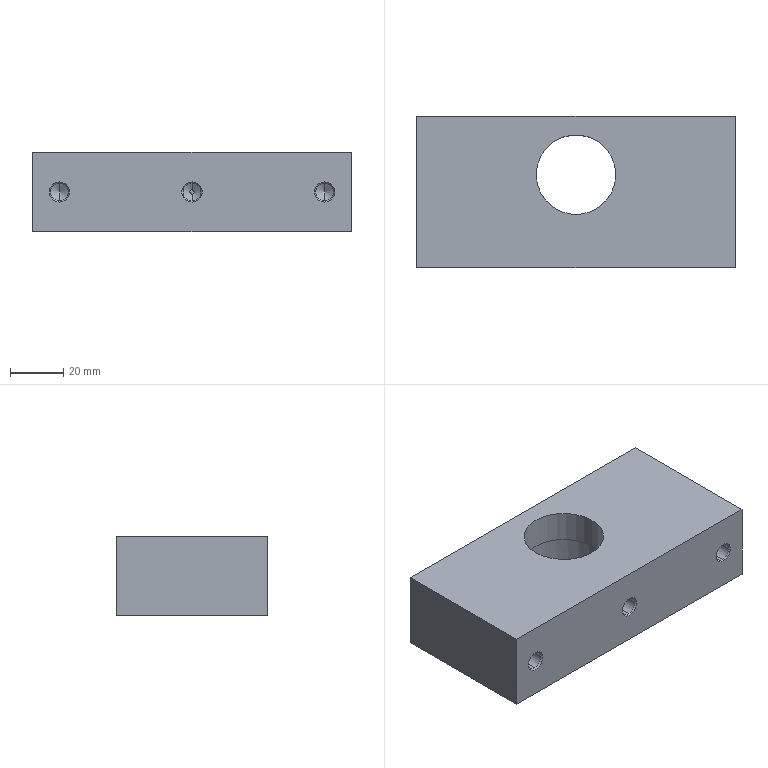Part | STEP file | Roller base 2 | 1 solid | 43 faces | box 120 x 57 x 30 mm | volume 174618 mm3 | cone 22 | cylinder 14 | plane 7 | commonest cylinder face diameters 6.647 x10 30 x2 37 x2